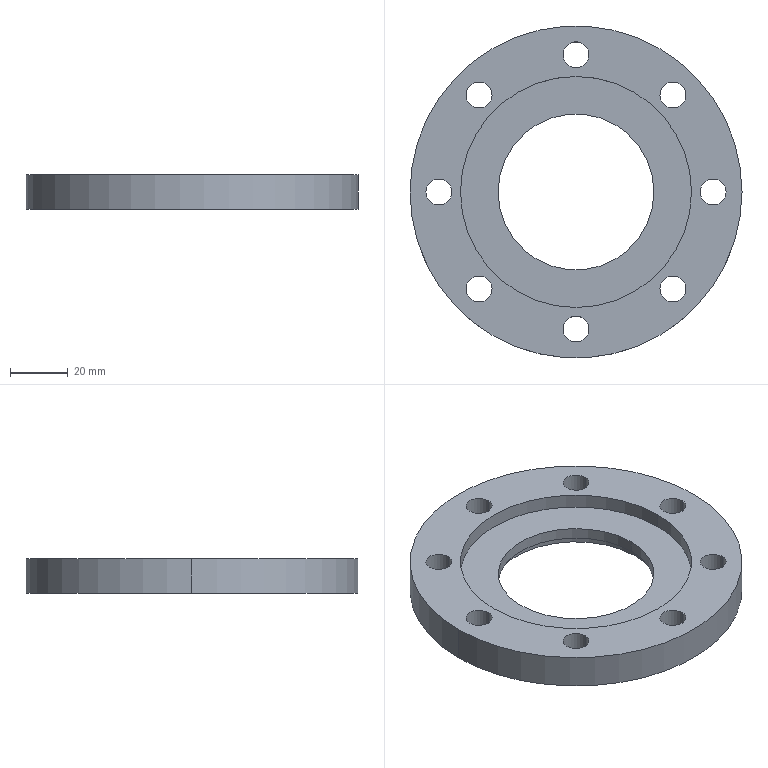Part | SolidWorks | features ICE 4, Extrusion 1 | 1 solid | 28 faces | box 115 x 115 x 12 mm | volume 76316 mm3 | cylinder 24 | plane 4 | commonest cylinder face diameters 9 x16 54 x2 58 x2 80 x2 115 x2
STEP:
#1=CARTESIAN_POINT('',(-4.5,47.5,0.));
#2=VERTEX_POINT('',#1);
#3=CARTESIAN_POINT('',(4.5,47.5,0.));
#4=VERTEX_POINT('',#3);
#5=CARTESIAN_POINT('',(0.,47.5,0.));
#6=DIRECTION('',(0.,0.,1.));
#7=DIRECTION('',(1.,0.,0.));
#8=AXIS2_PLACEMENT_3D('',#5,#6,#7);
#9=CIRCLE('',#8,4.5);
#10=EDGE_CURVE('',#2,#4,#9,.T.);
#11=ORIENTED_EDGE('',*,*,#10,.F.);
#12=CARTESIAN_POINT('',(-4.5,47.5,12.));
#13=VERTEX_POINT('',#12);
#14=CARTESIAN_POINT('',(-4.5,47.5,-38.));
#15=DIRECTION('',(0.,0.,1.));
#16=VECTOR('',#15,1000.);
#17=LINE('',#14,#16);
#18=EDGE_CURVE('',#2,#13,#17,.T.);
#19=ORIENTED_EDGE('',*,*,#18,.T.);
#20=CARTESIAN_POINT('',(4.5,47.5,12.));
#21=VERTEX_POINT('',#20);
#22=CARTESIAN_POINT('',(0.,47.5,12.));
#23=DIRECTION('',(0.,0.,1.));
#24=DIRECTION('',(1.,0.,0.));
#25=AXIS2_PLACEMENT_3D('',#22,#23,#24);
#26=CIRCLE('',#25,4.5);
#27=EDGE_CURVE('',#13,#21,#26,.T.);
#28=ORIENTED_EDGE('',*,*,#27,.T.);
#29=CARTESIAN_POINT('',(4.5,47.5,-38.));
#30=DIRECTION('',(0.,0.,1.));
#31=VECTOR('',#30,1000.);
#32=LINE('',#29,#31);
#33=EDGE_CURVE('',#4,#21,#32,.T.);
#34=ORIENTED_EDGE('',*,*,#33,.F.);
#35=EDGE_LOOP('',(#11,#19,#28,#34));
#36=FACE_OUTER_BOUND('',#35,.T.);
#37=CARTESIAN_POINT('',(0.,47.5,-38.));
#38=DIRECTION('',(0.,0.,1.));
#39=DIRECTION('',(1.,0.,0.));
#40=AXIS2_PLACEMENT_3D('',#37,#38,#39);
#41=CYLINDRICAL_SURFACE('',#40,4.5);
#42=ADVANCED_FACE('',(#36),#41,.F.);
#43=CARTESIAN_POINT('',(29.088,33.588,0.));
#44=VERTEX_POINT('',#43);
#45=CARTESIAN_POINT('',(38.088,33.588,0.));
#46=VERTEX_POINT('',#45);
#47=CARTESIAN_POINT('',(33.588,33.588,0.));
#48=DIRECTION('',(0.,0.,1.));
#49=DIRECTION('',(1.,0.,0.));
#50=AXIS2_PLACEMENT_3D('',#47,#48,#49);
#51=CIRCLE('',#50,4.5);
#52=EDGE_CURVE('',#44,#46,#51,.T.);
#53=ORIENTED_EDGE('',*,*,#52,.F.);
#54=CARTESIAN_POINT('',(29.088,33.588,12.));
#55=VERTEX_POINT('',#54);
#56=CARTESIAN_POINT('',(29.088,33.588,-38.));
#57=DIRECTION('',(0.,0.,1.));
#58=VECTOR('',#57,1000.);
#59=LINE('',#56,#58);
#60=EDGE_CURVE('',#44,#55,#59,.T.);
#61=ORIENTED_EDGE('',*,*,#60,.T.);
#62=CARTESIAN_POINT('',(38.088,33.588,12.));
#63=VERTEX_POINT('',#62);
#64=CARTESIAN_POINT('',(33.588,33.588,12.));
#65=DIRECTION('',(0.,0.,1.));
#66=DIRECTION('',(1.,0.,0.));
#67=AXIS2_PLACEMENT_3D('',#64,#65,#66);
#68=CIRCLE('',#67,4.5);
#69=EDGE_CURVE('',#55,#63,#68,.T.);
#70=ORIENTED_EDGE('',*,*,#69,.T.);
#71=CARTESIAN_POINT('',(38.088,33.588,-38.));
#72=DIRECTION('',(0.,0.,1.));
#73=VECTOR('',#72,1000.);
#74=LINE('',#71,#73);
#75=EDGE_CURVE('',#46,#63,#74,.T.);
#76=ORIENTED_EDGE('',*,*,#75,.F.);
#77=EDGE_LOOP('',(#53,#61,#70,#76));
#78=FACE_OUTER_BOUND('',#77,.T.);
#79=CARTESIAN_POINT('',(33.588,33.588,-38.));
#80=DIRECTION('',(0.,0.,1.));
#81=DIRECTION('',(1.,0.,0.));
#82=AXIS2_PLACEMENT_3D('',#79,#80,#81);
#83=CYLINDRICAL_SURFACE('',#82,4.5);
#84=ADVANCED_FACE('',(#78),#83,.F.);
#85=CARTESIAN_POINT('',(43.,0.,0.));
#86=VERTEX_POINT('',#85);
#87=CARTESIAN_POINT('',(52.,0.,0.));
#88=VERTEX_POINT('',#87);
#89=CARTESIAN_POINT('',(47.5,0.,0.));
#90=DIRECTION('',(0.,0.,1.));
#91=DIRECTION('',(1.,0.,0.));
#92=AXIS2_PLACEMENT_3D('',#89,#90,#91);
#93=CIRCLE('',#92,4.5);
#94=EDGE_CURVE('',#86,#88,#93,.T.);
#95=ORIENTED_EDGE('',*,*,#94,.F.);
#96=CARTESIAN_POINT('',(43.,0.,12.));
#97=VERTEX_POINT('',#96);
#98=CARTESIAN_POINT('',(43.,0.,-38.));
#99=DIRECTION('',(0.,0.,1.));
#100=VECTOR('',#99,1000.);
#101=LINE('',#98,#100);
#102=EDGE_CURVE('',#86,#97,#101,.T.);
#103=ORIENTED_EDGE('',*,*,#102,.T.);
#104=CARTESIAN_POINT('',(52.,0.,12.));
#105=VERTEX_POINT('',#104);
#106=CARTESIAN_POINT('',(47.5,0.,12.));
#107=DIRECTION('',(0.,0.,1.));
#108=DIRECTION('',(1.,0.,0.));
#109=AXIS2_PLACEMENT_3D('',#106,#107,#108);
#110=CIRCLE('',#109,4.5);
#111=EDGE_CURVE('',#97,#105,#110,.T.);
#112=ORIENTED_EDGE('',*,*,#111,.T.);
#113=CARTESIAN_POINT('',(52.,0.,-38.));
#114=DIRECTION('',(0.,0.,1.));
#115=VECTOR('',#114,1000.);
#116=LINE('',#113,#115);
#117=EDGE_CURVE('',#88,#105,#116,.T.);
#118=ORIENTED_EDGE('',*,*,#117,.F.);
#119=EDGE_LOOP('',(#95,#103,#112,#118));
#120=FACE_OUTER_BOUND('',#119,.T.);
#121=CARTESIAN_POINT('',(47.5,0.,-38.));
#122=DIRECTION('',(0.,0.,1.));
#123=DIRECTION('',(1.,0.,0.));
#124=AXIS2_PLACEMENT_3D('',#121,#122,#123);
#125=CYLINDRICAL_SURFACE('',#124,4.5);
#126=ADVANCED_FACE('',(#120),#125,.F.);
#127=CARTESIAN_POINT('',(29.088,-33.588,0.));
#128=VERTEX_POINT('',#127);
#129=CARTESIAN_POINT('',(38.088,-33.588,0.));
#130=VERTEX_POINT('',#129);
#131=CARTESIAN_POINT('',(33.588,-33.588,0.));
#132=DIRECTION('',(0.,0.,1.));
#133=DIRECTION('',(1.,0.,0.));
#134=AXIS2_PLACEMENT_3D('',#131,#132,#133);
#135=CIRCLE('',#134,4.5);
#136=EDGE_CURVE('',#128,#130,#135,.T.);
#137=ORIENTED_EDGE('',*,*,#136,.F.);
#138=CARTESIAN_POINT('',(29.088,-33.588,12.));
#139=VERTEX_POINT('',#138);
#140=CARTESIAN_POINT('',(29.088,-33.588,-38.));
#141=DIRECTION('',(0.,0.,1.));
#142=VECTOR('',#141,1000.);
#143=LINE('',#140,#142);
#144=EDGE_CURVE('',#128,#139,#143,.T.);
#145=ORIENTED_EDGE('',*,*,#144,.T.);
#146=CARTESIAN_POINT('',(38.088,-33.588,12.));
#147=VERTEX_POINT('',#146);
#148=CARTESIAN_POINT('',(33.588,-33.588,12.));
#149=DIRECTION('',(0.,0.,1.));
#150=DIRECTION('',(1.,0.,0.));
#151=AXIS2_PLACEMENT_3D('',#148,#149,#150);
#152=CIRCLE('',#151,4.5);
#153=EDGE_CURVE('',#139,#147,#152,.T.);
#154=ORIENTED_EDGE('',*,*,#153,.T.);
#155=CARTESIAN_POINT('',(38.088,-33.588,-38.));
#156=DIRECTION('',(0.,0.,1.));
#157=VECTOR('',#156,1000.);
#158=LINE('',#155,#157);
#159=EDGE_CURVE('',#130,#147,#158,.T.);
#160=ORIENTED_EDGE('',*,*,#159,.F.);
#161=EDGE_LOOP('',(#137,#145,#154,#160));
#162=FACE_OUTER_BOUND('',#161,.T.);
#163=CARTESIAN_POINT('',(33.588,-33.588,-38.));
#164=DIRECTION('',(0.,0.,1.));
#165=DIRECTION('',(1.,0.,0.));
#166=AXIS2_PLACEMENT_3D('',#163,#164,#165);
#167=CYLINDRICAL_SURFACE('',#166,4.5);
#168=ADVANCED_FACE('',(#162),#167,.F.);
#169=CARTESIAN_POINT('',(-4.5,-47.5,0.));
#170=VERTEX_POINT('',#169);
#171=CARTESIAN_POINT('',(4.5,-47.5,0.));
#172=VERTEX_POINT('',#171);
#173=CARTESIAN_POINT('',(0.,-47.5,0.));
#174=DIRECTION('',(0.,0.,1.));
#175=DIRECTION('',(1.,0.,0.));
#176=AXIS2_PLACEMENT_3D('',#173,#174,#175);
#177=CIRCLE('',#176,4.5);
#178=EDGE_CURVE('',#170,#172,#177,.T.);
#179=ORIENTED_EDGE('',*,*,#178,.F.);
#180=CARTESIAN_POINT('',(-4.5,-47.5,12.));
#181=VERTEX_POINT('',#180);
#182=CARTESIAN_POINT('',(-4.5,-47.5,-38.));
#183=DIRECTION('',(0.,0.,1.));
#184=VECTOR('',#183,1000.);
#185=LINE('',#182,#184);
#186=EDGE_CURVE('',#170,#181,#185,.T.);
#187=ORIENTED_EDGE('',*,*,#186,.T.);
#188=CARTESIAN_POINT('',(4.5,-47.5,12.));
#189=VERTEX_POINT('',#188);
#190=CARTESIAN_POINT('',(0.,-47.5,12.));
#191=DIRECTION('',(0.,0.,1.));
#192=DIRECTION('',(1.,0.,0.));
#193=AXIS2_PLACEMENT_3D('',#190,#191,#192);
#194=CIRCLE('',#193,4.5);
#195=EDGE_CURVE('',#181,#189,#194,.T.);
#196=ORIENTED_EDGE('',*,*,#195,.T.);
#197=CARTESIAN_POINT('',(4.5,-47.5,-38.));
#198=DIRECTION('',(0.,0.,1.));
#199=VECTOR('',#198,1000.);
#200=LINE('',#197,#199);
#201=EDGE_CURVE('',#172,#189,#200,.T.);
#202=ORIENTED_EDGE('',*,*,#201,.F.);
#203=EDGE_LOOP('',(#179,#187,#196,#202));
#204=FACE_OUTER_BOUND('',#203,.T.);
#205=CARTESIAN_POINT('',(0.,-47.5,-38.));
#206=DIRECTION('',(0.,0.,1.));
#207=DIRECTION('',(1.,0.,0.));
#208=AXIS2_PLACEMENT_3D('',#205,#206,#207);
#209=CYLINDRICAL_SURFACE('',#208,4.5);
#210=ADVANCED_FACE('',(#204),#209,.F.);
#211=CARTESIAN_POINT('',(-38.088,-33.588,0.));
#212=VERTEX_POINT('',#211);
#213=CARTESIAN_POINT('',(-29.088,-33.588,0.));
#214=VERTEX_POINT('',#213);
#215=CARTESIAN_POINT('',(-33.588,-33.588,0.));
#216=DIRECTION('',(0.,0.,1.));
#217=DIRECTION('',(1.,0.,0.));
#218=AXIS2_PLACEMENT_3D('',#215,#216,#217);
#219=CIRCLE('',#218,4.5);
#220=EDGE_CURVE('',#212,#214,#219,.T.);
#221=ORIENTED_EDGE('',*,*,#220,.F.);
#222=CARTESIAN_POINT('',(-38.088,-33.588,12.));
#223=VERTEX_POINT('',#222);
#224=CARTESIAN_POINT('',(-38.088,-33.588,-38.));
#225=DIRECTION('',(0.,0.,1.));
#226=VECTOR('',#225,1000.);
#227=LINE('',#224,#226);
#228=EDGE_CURVE('',#212,#223,#227,.T.);
#229=ORIENTED_EDGE('',*,*,#228,.T.);
#230=CARTESIAN_POINT('',(-29.088,-33.588,12.));
#231=VERTEX_POINT('',#230);
#232=CARTESIAN_POINT('',(-33.588,-33.588,12.));
#233=DIRECTION('',(0.,0.,1.));
#234=DIRECTION('',(1.,0.,0.));
#235=AXIS2_PLACEMENT_3D('',#232,#233,#234);
#236=CIRCLE('',#235,4.5);
#237=EDGE_CURVE('',#223,#231,#236,.T.);
#238=ORIENTED_EDGE('',*,*,#237,.T.);
#239=CARTESIAN_POINT('',(-29.088,-33.588,-38.));
#240=DIRECTION('',(0.,0.,1.));
#241=VECTOR('',#240,1000.);
#242=LINE('',#239,#241);
#243=EDGE_CURVE('',#214,#231,#242,.T.);
#244=ORIENTED_EDGE('',*,*,#243,.F.);
#245=EDGE_LOOP('',(#221,#229,#238,#244));
#246=FACE_OUTER_BOUND('',#245,.T.);
#247=CARTESIAN_POINT('',(-33.588,-33.588,-38.));
#248=DIRECTION('',(0.,0.,1.));
#249=DIRECTION('',(1.,0.,0.));
#250=AXIS2_PLACEMENT_3D('',#247,#248,#249);
#251=CYLINDRICAL_SURFACE('',#250,4.5);
#252=ADVANCED_FACE('',(#246),#251,.F.);
#253=CARTESIAN_POINT('',(-52.,0.,0.));
#254=VERTEX_POINT('',#253);
#255=CARTESIAN_POINT('',(-43.,0.,0.));
#256=VERTEX_POINT('',#255);
#257=CARTESIAN_POINT('',(-47.5,0.,0.));
#258=DIRECTION('',(0.,0.,1.));
#259=DIRECTION('',(1.,0.,0.));
#260=AXIS2_PLACEMENT_3D('',#257,#258,#259);
#261=CIRCLE('',#260,4.5);
#262=EDGE_CURVE('',#254,#256,#261,.T.);
#263=ORIENTED_EDGE('',*,*,#262,.F.);
#264=CARTESIAN_POINT('',(-52.,0.,12.));
#265=VERTEX_POINT('',#264);
#266=CARTESIAN_POINT('',(-52.,0.,-38.));
#267=DIRECTION('',(0.,0.,1.));
#268=VECTOR('',#267,1000.);
#269=LINE('',#266,#268);
#270=EDGE_CURVE('',#254,#265,#269,.T.);
#271=ORIENTED_EDGE('',*,*,#270,.T.);
#272=CARTESIAN_POINT('',(-43.,0.,12.));
#273=VERTEX_POINT('',#272);
#274=CARTESIAN_POINT('',(-47.5,0.,12.));
#275=DIRECTION('',(0.,0.,1.));
#276=DIRECTION('',(1.,0.,0.));
#277=AXIS2_PLACEMENT_3D('',#274,#275,#276);
#278=CIRCLE('',#277,4.5);
#279=EDGE_CURVE('',#265,#273,#278,.T.);
#280=ORIENTED_EDGE('',*,*,#279,.T.);
#281=CARTESIAN_POINT('',(-43.,0.,-38.));
#282=DIRECTION('',(0.,0.,1.));
#283=VECTOR('',#282,1000.);
#284=LINE('',#281,#283);
#285=EDGE_CURVE('',#256,#273,#284,.T.);
#286=ORIENTED_EDGE('',*,*,#285,.F.);
#287=EDGE_LOOP('',(#263,#271,#280,#286));
#288=FACE_OUTER_BOUND('',#287,.T.);
#289=CARTESIAN_POINT('',(-47.5,0.,-38.));
#290=DIRECTION('',(0.,0.,1.));
#291=DIRECTION('',(1.,0.,0.));
#292=AXIS2_PLACEMENT_3D('',#289,#290,#291);
#293=CYLINDRICAL_SURFACE('',#292,4.5);
#294=ADVANCED_FACE('',(#288),#293,.F.);
#295=CARTESIAN_POINT('',(-38.088,33.588,0.));
#296=VERTEX_POINT('',#295);
#297=CARTESIAN_POINT('',(-29.088,33.588,0.));
#298=VERTEX_POINT('',#297);
#299=CARTESIAN_POINT('',(-33.588,33.588,0.));
#300=DIRECTION('',(0.,0.,1.));
#301=DIRECTION('',(1.,0.,0.));
#302=AXIS2_PLACEMENT_3D('',#299,#300,#301);
#303=CIRCLE('',#302,4.5);
#304=EDGE_CURVE('',#296,#298,#303,.T.);
#305=ORIENTED_EDGE('',*,*,#304,.F.);
#306=CARTESIAN_POINT('',(-38.088,33.588,12.));
#307=VERTEX_POINT('',#306);
#308=CARTESIAN_POINT('',(-38.088,33.588,-38.));
#309=DIRECTION('',(0.,0.,1.));
#310=VECTOR('',#309,1000.);
#311=LINE('',#308,#310);
#312=EDGE_CURVE('',#296,#307,#311,.T.);
#313=ORIENTED_EDGE('',*,*,#312,.T.);
#314=CARTESIAN_POINT('',(-29.088,33.588,12.));
#315=VERTEX_POINT('',#314);
#316=CARTESIAN_POINT('',(-33.588,33.588,12.));
#317=DIRECTION('',(0.,0.,1.));
#318=DIRECTION('',(1.,0.,0.));
#319=AXIS2_PLACEMENT_3D('',#316,#317,#318);
#320=CIRCLE('',#319,4.5);
#321=EDGE_CURVE('',#307,#315,#320,.T.);
#322=ORIENTED_EDGE('',*,*,#321,.T.);
#323=CARTESIAN_POINT('',(-29.088,33.588,-38.));
#324=DIRECTION('',(0.,0.,1.));
#325=VECTOR('',#324,1000.);
#326=LINE('',#323,#325);
#327=EDGE_CURVE('',#298,#315,#326,.T.);
#328=ORIENTED_EDGE('',*,*,#327,.F.);
#329=EDGE_LOOP('',(#305,#313,#322,#328));
#330=FACE_OUTER_BOUND('',#329,.T.);
#331=CARTESIAN_POINT('',(-33.588,33.588,-38.));
#332=DIRECTION('',(0.,0.,1.));
#333=DIRECTION('',(1.,0.,0.));
#334=AXIS2_PLACEMENT_3D('',#331,#332,#333);
#335=CYLINDRICAL_SURFACE('',#334,4.5);
#336=ADVANCED_FACE('',(#330),#335,.F.);
#337=CARTESIAN_POINT('',(29.,0.,3.));
#338=VERTEX_POINT('',#337);
#339=CARTESIAN_POINT('',(-29.,0.,3.));
#340=VERTEX_POINT('',#339);
#341=CARTESIAN_POINT('',(0.,0.,3.));
#342=DIRECTION('',(0.,0.,-1.));
#343=DIRECTION('',(-1.,0.,0.));
#344=AXIS2_PLACEMENT_3D('',#341,#342,#343);
#345=CIRCLE('',#344,29.);
#346=EDGE_CURVE('',#338,#340,#345,.T.);
#347=ORIENTED_EDGE('',*,*,#346,.F.);
#348=CARTESIAN_POINT('',(29.,0.,0.));
#349=VERTEX_POINT('',#348);
#350=CARTESIAN_POINT('',(29.,0.,3.));
#351=DIRECTION('',(0.,0.,-1.));
#352=VECTOR('',#351,1000.);
#353=LINE('',#350,#352);
#354=EDGE_CURVE('',#338,#349,#353,.T.);
#355=ORIENTED_EDGE('',*,*,#354,.T.);
#356=CARTESIAN_POINT('',(-29.,0.,0.));
#357=VERTEX_POINT('',#356);
#358=CARTESIAN_POINT('',(0.,0.,0.));
#359=DIRECTION('',(0.,0.,-1.));
#360=DIRECTION('',(-1.,0.,0.));
#361=AXIS2_PLACEMENT_3D('',#358,#359,#360);
#362=CIRCLE('',#361,29.);
#363=EDGE_CURVE('',#349,#357,#362,.T.);
#364=ORIENTED_EDGE('',*,*,#363,.T.);
#365=CARTESIAN_POINT('',(-29.,0.,3.));
#366=DIRECTION('',(0.,0.,-1.));
#367=VECTOR('',#366,1000.);
#368=LINE('',#365,#367);
#369=EDGE_CURVE('',#340,#357,#368,.T.);
#370=ORIENTED_EDGE('',*,*,#369,.F.);
#371=EDGE_LOOP('',(#347,#355,#364,#370));
#372=FACE_OUTER_BOUND('',#371,.T.);
#373=CARTESIAN_POINT('',(0.,0.,3.));
#374=DIRECTION('',(0.,0.,-1.));
#375=DIRECTION('',(-1.,0.,0.));
#376=AXIS2_PLACEMENT_3D('',#373,#374,#375);
#377=CYLINDRICAL_SURFACE('',#376,29.);
#378=ADVANCED_FACE('',(#372),#377,.F.);
#379=CARTESIAN_POINT('',(-40.,0.,7.));
#380=VERTEX_POINT('',#379);
#381=CARTESIAN_POINT('',(40.,0.,7.));
#382=VERTEX_POINT('',#381);
#383=CARTESIAN_POINT('',(0.,0.,7.));
#384=DIRECTION('',(0.,0.,1.));
#385=DIRECTION('',(1.,0.,0.));
#386=AXIS2_PLACEMENT_3D('',#383,#384,#385);
#387=CIRCLE('',#386,40.);
#388=EDGE_CURVE('',#380,#382,#387,.T.);
#389=ORIENTED_EDGE('',*,*,#388,.F.);
#390=CARTESIAN_POINT('',(-40.,0.,12.));
#391=VERTEX_POINT('',#390);
#392=CARTESIAN_POINT('',(-40.,0.,7.));
#393=DIRECTION('',(0.,0.,1.));
#394=VECTOR('',#393,1000.);
#395=LINE('',#392,#394);
#396=EDGE_CURVE('',#380,#391,#395,.T.);
#397=ORIENTED_EDGE('',*,*,#396,.T.);
#398=CARTESIAN_POINT('',(40.,0.,12.));
#399=VERTEX_POINT('',#398);
#400=CARTESIAN_POINT('',(0.,0.,12.));
#401=DIRECTION('',(0.,0.,1.));
#402=DIRECTION('',(1.,0.,0.));
#403=AXIS2_PLACEMENT_3D('',#400,#401,#402);
#404=CIRCLE('',#403,40.);
#405=EDGE_CURVE('',#391,#399,#404,.T.);
#406=ORIENTED_EDGE('',*,*,#405,.T.);
#407=CARTESIAN_POINT('',(40.,0.,7.));
#408=DIRECTION('',(0.,0.,1.));
#409=VECTOR('',#408,1000.);
#410=LINE('',#407,#409);
#411=EDGE_CURVE('',#382,#399,#410,.T.);
#412=ORIENTED_EDGE('',*,*,#411,.F.);
#413=EDGE_LOOP('',(#389,#397,#406,#412));
#414=FACE_OUTER_BOUND('',#413,.T.);
#415=CARTESIAN_POINT('',(0.,0.,7.));
#416=DIRECTION('',(0.,0.,1.));
#417=DIRECTION('',(1.,0.,0.));
#418=AXIS2_PLACEMENT_3D('',#415,#416,#417);
#419=CYLINDRICAL_SURFACE('',#418,40.);
#420=ADVANCED_FACE('',(#414),#419,.F.);
#421=CARTESIAN_POINT('',(57.5,0.,12.));
#422=VERTEX_POINT('',#421);
#423=CARTESIAN_POINT('',(-57.5,0.,12.));
#424=VERTEX_POINT('',#423);
#425=CARTESIAN_POINT('',(0.,0.,12.));
#426=DIRECTION('',(0.,0.,1.));
#427=DIRECTION('',(1.,0.,0.));
#428=AXIS2_PLACEMENT_3D('',#425,#426,#427);
#429=CIRCLE('',#428,57.5);
#430=EDGE_CURVE('',#422,#424,#429,.T.);
#431=ORIENTED_EDGE('',*,*,#430,.F.);
#432=CARTESIAN_POINT('',(57.5,0.,0.));
#433=VERTEX_POINT('',#432);
#434=CARTESIAN_POINT('',(57.5,0.,12.));
#435=DIRECTION('',(0.,0.,-1.));
#436=VECTOR('',#435,1000.);
#437=LINE('',#434,#436);
#438=EDGE_CURVE('',#422,#433,#437,.T.);
#439=ORIENTED_EDGE('',*,*,#438,.T.);
#440=CARTESIAN_POINT('',(-57.5,0.,0.));
#441=VERTEX_POINT('',#440);
#442=CARTESIAN_POINT('',(0.,0.,0.));
#443=DIRECTION('',(0.,0.,1.));
#444=DIRECTION('',(1.,0.,0.));
#445=AXIS2_PLACEMENT_3D('',#442,#443,#444);
#446=CIRCLE('',#445,57.5);
#447=EDGE_CURVE('',#433,#441,#446,.T.);
#448=ORIENTED_EDGE('',*,*,#447,.T.);
#449=CARTESIAN_POINT('',(-57.5,0.,12.));
#450=DIRECTION('',(0.,0.,-1.));
#451=VECTOR('',#450,1000.);
#452=LINE('',#449,#451);
#453=EDGE_CURVE('',#424,#441,#452,.T.);
#454=ORIENTED_EDGE('',*,*,#453,.F.);
#455=EDGE_LOOP('',(#431,#439,#448,#454));
#456=FACE_OUTER_BOUND('',#455,.T.);
#457=CARTESIAN_POINT('',(0.,0.,12.));
#458=DIRECTION('',(0.,0.,-1.));
#459=DIRECTION('',(-1.,0.,0.));
#460=AXIS2_PLACEMENT_3D('',#457,#458,#459);
#461=CYLINDRICAL_SURFACE('',#460,57.5);
#462=ADVANCED_FACE('',(#456),#461,.T.);
#463=CARTESIAN_POINT('',(-27.,0.,3.));
#464=VERTEX_POINT('',#463);
#465=CARTESIAN_POINT('',(27.,0.,3.));
#466=VERTEX_POINT('',#465);
#467=CARTESIAN_POINT('',(0.,0.,3.));
#468=DIRECTION('',(0.,0.,1.));
#469=DIRECTION('',(-1.,0.,0.));
#470=AXIS2_PLACEMENT_3D('',#467,#468,#469);
#471=CIRCLE('',#470,27.);
#472=EDGE_CURVE('',#464,#466,#471,.T.);
#473=ORIENTED_EDGE('',*,*,#472,.F.);
#474=CARTESIAN_POINT('',(-27.,0.,7.));
#475=VERTEX_POINT('',#474);
#476=CARTESIAN_POINT('',(-27.,0.,-6.));
#477=DIRECTION('',(0.,0.,1.));
#478=VECTOR('',#477,1000.);
#479=LINE('',#476,#478);
#480=EDGE_CURVE('',#464,#475,#479,.T.);
#481=ORIENTED_EDGE('',*,*,#480,.T.);
#482=CARTESIAN_POINT('',(27.,0.,7.));
#483=VERTEX_POINT('',#482);
#484=CARTESIAN_POINT('',(0.,0.,7.));
#485=DIRECTION('',(0.,0.,1.));
#486=DIRECTION('',(1.,0.,0.));
#487=AXIS2_PLACEMENT_3D('',#484,#485,#486);
#488=CIRCLE('',#487,27.);
#489=EDGE_CURVE('',#475,#483,#488,.T.);
#490=ORIENTED_EDGE('',*,*,#489,.T.);
#491=CARTESIAN_POINT('',(27.,0.,-6.));
#492=DIRECTION('',(0.,0.,1.));
#493=VECTOR('',#492,1000.);
#494=LINE('',#491,#493);
#495=EDGE_CURVE('',#466,#483,#494,.T.);
#496=ORIENTED_EDGE('',*,*,#495,.F.);
#497=EDGE_LOOP('',(#473,#481,#490,#496));
#498=FACE_OUTER_BOUND('',#497,.T.);
#499=CARTESIAN_POINT('',(0.,0.,-6.));
#500=DIRECTION('',(0.,0.,1.));
#501=DIRECTION('',(1.,0.,0.));
#502=AXIS2_PLACEMENT_3D('',#499,#500,#501);
#503=CYLINDRICAL_SURFACE('',#502,27.);
#504=ADVANCED_FACE('',(#498),#503,.F.);
#505=ORIENTED_EDGE('',*,*,#480,.F.);
#506=CARTESIAN_POINT('',(0.,0.,3.));
#507=DIRECTION('',(0.,0.,1.));
#508=DIRECTION('',(-1.,0.,0.));
#509=AXIS2_PLACEMENT_3D('',#506,#507,#508);
#510=CIRCLE('',#509,27.);
#511=EDGE_CURVE('',#466,#464,#510,.T.);
#512=ORIENTED_EDGE('',*,*,#511,.F.);
#513=ORIENTED_EDGE('',*,*,#495,.T.);
#514=CARTESIAN_POINT('',(0.,0.,7.));
#515=DIRECTION('',(0.,0.,1.));
#516=DIRECTION('',(1.,0.,0.));
#517=AXIS2_PLACEMENT_3D('',#514,#515,#516);
#518=CIRCLE('',#517,27.);
#519=EDGE_CURVE('',#483,#475,#518,.T.);
#520=ORIENTED_EDGE('',*,*,#519,.T.);
#521=EDGE_LOOP('',(#505,#512,#513,#520));
#522=FACE_OUTER_BOUND('',#521,.T.);
#523=CARTESIAN_POINT('',(0.,0.,-6.));
#524=DIRECTION('',(0.,0.,1.));
#525=DIRECTION('',(1.,0.,0.));
#526=AXIS2_PLACEMENT_3D('',#523,#524,#525);
#527=CYLINDRICAL_SURFACE('',#526,27.);
#528=ADVANCED_FACE('',(#522),#527,.F.);
#529=ORIENTED_EDGE('',*,*,#438,.F.);
#530=CARTESIAN_POINT('',(0.,0.,12.));
#531=DIRECTION('',(0.,0.,1.));
#532=DIRECTION('',(1.,0.,0.));
#533=AXIS2_PLACEMENT_3D('',#530,#531,#532);
#534=CIRCLE('',#533,57.5);
#535=EDGE_CURVE('',#424,#422,#534,.T.);
#536=ORIENTED_EDGE('',*,*,#535,.F.);
#537=ORIENTED_EDGE('',*,*,#453,.T.);
#538=CARTESIAN_POINT('',(0.,0.,0.));
#539=DIRECTION('',(0.,0.,1.));
#540=DIRECTION('',(1.,0.,0.));
#541=AXIS2_PLACEMENT_3D('',#538,#539,#540);
#542=CIRCLE('',#541,57.5);
#543=EDGE_CURVE('',#441,#433,#542,.T.);
#544=ORIENTED_EDGE('',*,*,#543,.T.);
#545=EDGE_LOOP('',(#529,#536,#537,#544));
#546=FACE_OUTER_BOUND('',#545,.T.);
#547=CARTESIAN_POINT('',(0.,0.,12.));
#548=DIRECTION('',(0.,0.,-1.));
#549=DIRECTION('',(-1.,0.,0.));
#550=AXIS2_PLACEMENT_3D('',#547,#548,#549);
#551=CYLINDRICAL_SURFACE('',#550,57.5);
#552=ADVANCED_FACE('',(#546),#551,.T.);
#553=CARTESIAN_POINT('',(0.,47.5,12.));
#554=DIRECTION('',(0.,0.,1.));
#555=DIRECTION('',(1.,0.,0.));
#556=AXIS2_PLACEMENT_3D('',#553,#554,#555);
#557=CIRCLE('',#556,4.5);
#558=EDGE_CURVE('',#21,#13,#557,.T.);
#559=ORIENTED_EDGE('',*,*,#558,.F.);
#560=ORIENTED_EDGE('',*,*,#27,.F.);
#561=EDGE_LOOP('',(#559,#560));
#562=FACE_BOUND('',#561,.T.);
#563=CARTESIAN_POINT('',(33.588,33.588,12.));
#564=DIRECTION('',(0.,0.,1.));
#565=DIRECTION('',(1.,0.,0.));
#566=AXIS2_PLACEMENT_3D('',#563,#564,#565);
#567=CIRCLE('',#566,4.5);
#568=EDGE_CURVE('',#63,#55,#567,.T.);
#569=ORIENTED_EDGE('',*,*,#568,.F.);
#570=ORIENTED_EDGE('',*,*,#69,.F.);
#571=EDGE_LOOP('',(#569,#570));
#572=FACE_BOUND('',#571,.T.);
#573=CARTESIAN_POINT('',(47.5,0.,12.));
#574=DIRECTION('',(0.,0.,1.));
#575=DIRECTION('',(1.,0.,0.));
#576=AXIS2_PLACEMENT_3D('',#573,#574,#575);
#577=CIRCLE('',#576,4.5);
#578=EDGE_CURVE('',#105,#97,#577,.T.);
#579=ORIENTED_EDGE('',*,*,#578,.F.);
#580=ORIENTED_EDGE('',*,*,#111,.F.);
#581=EDGE_LOOP('',(#579,#580));
#582=FACE_BOUND('',#581,.T.);
#583=CARTESIAN_POINT('',(33.588,-33.588,12.));
#584=DIRECTION('',(0.,0.,1.));
#585=DIRECTION('',(1.,0.,0.));
#586=AXIS2_PLACEMENT_3D('',#583,#584,#585);
#587=CIRCLE('',#586,4.5);
#588=EDGE_CURVE('',#147,#139,#587,.T.);
#589=ORIENTED_EDGE('',*,*,#588,.F.);
#590=ORIENTED_EDGE('',*,*,#153,.F.);
#591=EDGE_LOOP('',(#589,#590));
#592=FACE_BOUND('',#591,.T.);
#593=CARTESIAN_POINT('',(0.,-47.5,12.));
#594=DIRECTION('',(0.,0.,1.));
#595=DIRECTION('',(1.,0.,0.));
#596=AXIS2_PLACEMENT_3D('',#593,#594,#595);
#597=CIRCLE('',#596,4.5);
#598=EDGE_CURVE('',#189,#181,#597,.T.);
#599=ORIENTED_EDGE('',*,*,#598,.F.);
#600=ORIENTED_EDGE('',*,*,#195,.F.);
#601=EDGE_LOOP('',(#599,#600));
#602=FACE_BOUND('',#601,.T.);
#603=CARTESIAN_POINT('',(-33.588,-33.588,12.));
#604=DIRECTION('',(0.,0.,1.));
#605=DIRECTION('',(1.,0.,0.));
#606=AXIS2_PLACEMENT_3D('',#603,#604,#605);
#607=CIRCLE('',#606,4.5);
#608=EDGE_CURVE('',#231,#223,#607,.T.);
#609=ORIENTED_EDGE('',*,*,#608,.F.);
#610=ORIENTED_EDGE('',*,*,#237,.F.);
#611=EDGE_LOOP('',(#609,#610));
#612=FACE_BOUND('',#611,.T.);
#613=CARTESIAN_POINT('',(-47.5,0.,12.));
#614=DIRECTION('',(0.,0.,1.));
#615=DIRECTION('',(1.,0.,0.));
#616=AXIS2_PLACEMENT_3D('',#613,#614,#615);
#617=CIRCLE('',#616,4.5);
#618=EDGE_CURVE('',#273,#265,#617,.T.);
#619=ORIENTED_EDGE('',*,*,#618,.F.);
#620=ORIENTED_EDGE('',*,*,#279,.F.);
#621=EDGE_LOOP('',(#619,#620));
#622=FACE_BOUND('',#621,.T.);
#623=CARTESIAN_POINT('',(-33.588,33.588,12.));
#624=DIRECTION('',(0.,0.,1.));
#625=DIRECTION('',(1.,0.,0.));
#626=AXIS2_PLACEMENT_3D('',#623,#624,#625);
#627=CIRCLE('',#626,4.5);
#628=EDGE_CURVE('',#315,#307,#627,.T.);
#629=ORIENTED_EDGE('',*,*,#628,.F.);
#630=ORIENTED_EDGE('',*,*,#321,.F.);
#631=EDGE_LOOP('',(#629,#630));
#632=FACE_BOUND('',#631,.T.);
#633=CARTESIAN_POINT('',(0.,0.,12.));
#634=DIRECTION('',(0.,0.,1.));
#635=DIRECTION('',(1.,0.,0.));
#636=AXIS2_PLACEMENT_3D('',#633,#634,#635);
#637=CIRCLE('',#636,40.);
#638=EDGE_CURVE('',#399,#391,#637,.T.);
#639=ORIENTED_EDGE('',*,*,#638,.F.);
#640=ORIENTED_EDGE('',*,*,#405,.F.);
#641=EDGE_LOOP('',(#639,#640));
#642=FACE_BOUND('',#641,.T.);
#643=ORIENTED_EDGE('',*,*,#535,.T.);
#644=ORIENTED_EDGE('',*,*,#430,.T.);
#645=EDGE_LOOP('',(#643,#644));
#646=FACE_OUTER_BOUND('',#645,.T.);
#647=CARTESIAN_POINT('',(0.,0.,12.));
#648=DIRECTION('',(0.,0.,1.));
#649=DIRECTION('',(1.,0.,0.));
#650=AXIS2_PLACEMENT_3D('',#647,#648,#649);
#651=PLANE('',#650);
#652=ADVANCED_FACE('',(#562,#572,#582,#592,#602,#612,#622,#632,#642,#646),#651,.T.);
#653=CARTESIAN_POINT('',(0.,47.5,0.));
#654=DIRECTION('',(0.,0.,1.));
#655=DIRECTION('',(1.,0.,0.));
#656=AXIS2_PLACEMENT_3D('',#653,#654,#655);
#657=CIRCLE('',#656,4.5);
#658=EDGE_CURVE('',#4,#2,#657,.T.);
#659=ORIENTED_EDGE('',*,*,#658,.T.);
#660=ORIENTED_EDGE('',*,*,#10,.T.);
#661=EDGE_LOOP('',(#659,#660));
#662=FACE_BOUND('',#661,.T.);
#663=CARTESIAN_POINT('',(33.588,33.588,0.));
#664=DIRECTION('',(0.,0.,1.));
#665=DIRECTION('',(1.,0.,0.));
#666=AXIS2_PLACEMENT_3D('',#663,#664,#665);
#667=CIRCLE('',#666,4.5);
#668=EDGE_CURVE('',#46,#44,#667,.T.);
#669=ORIENTED_EDGE('',*,*,#668,.T.);
#670=ORIENTED_EDGE('',*,*,#52,.T.);
#671=EDGE_LOOP('',(#669,#670));
#672=FACE_BOUND('',#671,.T.);
#673=CARTESIAN_POINT('',(47.5,0.,0.));
#674=DIRECTION('',(0.,0.,1.));
#675=DIRECTION('',(1.,0.,0.));
#676=AXIS2_PLACEMENT_3D('',#673,#674,#675);
#677=CIRCLE('',#676,4.5);
#678=EDGE_CURVE('',#88,#86,#677,.T.);
#679=ORIENTED_EDGE('',*,*,#678,.T.);
#680=ORIENTED_EDGE('',*,*,#94,.T.);
#681=EDGE_LOOP('',(#679,#680));
#682=FACE_BOUND('',#681,.T.);
#683=CARTESIAN_POINT('',(33.588,-33.588,0.));
#684=DIRECTION('',(0.,0.,1.));
#685=DIRECTION('',(1.,0.,0.));
#686=AXIS2_PLACEMENT_3D('',#683,#684,#685);
#687=CIRCLE('',#686,4.5);
#688=EDGE_CURVE('',#130,#128,#687,.T.);
#689=ORIENTED_EDGE('',*,*,#688,.T.);
#690=ORIENTED_EDGE('',*,*,#136,.T.);
#691=EDGE_LOOP('',(#689,#690));
#692=FACE_BOUND('',#691,.T.);
#693=CARTESIAN_POINT('',(0.,-47.5,0.));
#694=DIRECTION('',(0.,0.,1.));
#695=DIRECTION('',(1.,0.,0.));
#696=AXIS2_PLACEMENT_3D('',#693,#694,#695);
#697=CIRCLE('',#696,4.5);
#698=EDGE_CURVE('',#172,#170,#697,.T.);
#699=ORIENTED_EDGE('',*,*,#698,.T.);
#700=ORIENTED_EDGE('',*,*,#178,.T.);
#701=EDGE_LOOP('',(#699,#700));
#702=FACE_BOUND('',#701,.T.);
#703=CARTESIAN_POINT('',(-33.588,-33.588,0.));
#704=DIRECTION('',(0.,0.,1.));
#705=DIRECTION('',(1.,0.,0.));
#706=AXIS2_PLACEMENT_3D('',#703,#704,#705);
#707=CIRCLE('',#706,4.5);
#708=EDGE_CURVE('',#214,#212,#707,.T.);
#709=ORIENTED_EDGE('',*,*,#708,.T.);
#710=ORIENTED_EDGE('',*,*,#220,.T.);
#711=EDGE_LOOP('',(#709,#710));
#712=FACE_BOUND('',#711,.T.);
#713=CARTESIAN_POINT('',(-47.5,0.,0.));
#714=DIRECTION('',(0.,0.,1.));
#715=DIRECTION('',(1.,0.,0.));
#716=AXIS2_PLACEMENT_3D('',#713,#714,#715);
#717=CIRCLE('',#716,4.5);
#718=EDGE_CURVE('',#256,#254,#717,.T.);
#719=ORIENTED_EDGE('',*,*,#718,.T.);
#720=ORIENTED_EDGE('',*,*,#262,.T.);
#721=EDGE_LOOP('',(#719,#720));
#722=FACE_BOUND('',#721,.T.);
#723=CARTESIAN_POINT('',(-33.588,33.588,0.));
#724=DIRECTION('',(0.,0.,1.));
#725=DIRECTION('',(1.,0.,0.));
#726=AXIS2_PLACEMENT_3D('',#723,#724,#725);
#727=CIRCLE('',#726,4.5);
#728=EDGE_CURVE('',#298,#296,#727,.T.);
#729=ORIENTED_EDGE('',*,*,#728,.T.);
#730=ORIENTED_EDGE('',*,*,#304,.T.);
#731=EDGE_LOOP('',(#729,#730));
#732=FACE_BOUND('',#731,.T.);
#733=CARTESIAN_POINT('',(0.,0.,0.));
#734=DIRECTION('',(0.,0.,-1.));
#735=DIRECTION('',(-1.,0.,0.));
#736=AXIS2_PLACEMENT_3D('',#733,#734,#735);
#737=CIRCLE('',#736,29.);
#738=EDGE_CURVE('',#357,#349,#737,.T.);
#739=ORIENTED_EDGE('',*,*,#738,.F.);
#740=ORIENTED_EDGE('',*,*,#363,.F.);
#741=EDGE_LOOP('',(#739,#740));
#742=FACE_BOUND('',#741,.T.);
#743=ORIENTED_EDGE('',*,*,#543,.F.);
#744=ORIENTED_EDGE('',*,*,#447,.F.);
#745=EDGE_LOOP('',(#743,#744));
#746=FACE_OUTER_BOUND('',#745,.T.);
#747=CARTESIAN_POINT('',(0.,0.,0.));
#748=DIRECTION('',(0.,0.,1.));
#749=DIRECTION('',(1.,0.,0.));
#750=AXIS2_PLACEMENT_3D('',#747,#748,#749);
#751=PLANE('',#750);
#752=ADVANCED_FACE('',(#662,#672,#682,#692,#702,#712,#722,#732,#742,#746),#751,.F.);
#753=ORIENTED_EDGE('',*,*,#396,.F.);
#754=CARTESIAN_POINT('',(0.,0.,7.));
#755=DIRECTION('',(0.,0.,1.));
#756=DIRECTION('',(1.,0.,0.));
#757=AXIS2_PLACEMENT_3D('',#754,#755,#756);
#758=CIRCLE('',#757,40.);
#759=EDGE_CURVE('',#382,#380,#758,.T.);
#760=ORIENTED_EDGE('',*,*,#759,.F.);
#761=ORIENTED_EDGE('',*,*,#411,.T.);
#762=ORIENTED_EDGE('',*,*,#638,.T.);
#763=EDGE_LOOP('',(#753,#760,#761,#762));
#764=FACE_OUTER_BOUND('',#763,.T.);
#765=CARTESIAN_POINT('',(0.,0.,7.));
#766=DIRECTION('',(0.,0.,1.));
#767=DIRECTION('',(1.,0.,0.));
#768=AXIS2_PLACEMENT_3D('',#765,#766,#767);
#769=CYLINDRICAL_SURFACE('',#768,40.);
#770=ADVANCED_FACE('',(#764),#769,.F.);
#771=ORIENTED_EDGE('',*,*,#519,.F.);
#772=ORIENTED_EDGE('',*,*,#489,.F.);
#773=EDGE_LOOP('',(#771,#772));
#774=FACE_BOUND('',#773,.T.);
#775=ORIENTED_EDGE('',*,*,#759,.T.);
#776=ORIENTED_EDGE('',*,*,#388,.T.);
#777=EDGE_LOOP('',(#775,#776));
#778=FACE_OUTER_BOUND('',#777,.T.);
#779=CARTESIAN_POINT('',(0.,0.,7.));
#780=DIRECTION('',(0.,0.,1.));
#781=DIRECTION('',(1.,0.,0.));
#782=AXIS2_PLACEMENT_3D('',#779,#780,#781);
#783=PLANE('',#782);
#784=ADVANCED_FACE('',(#774,#778),#783,.T.);
#785=CARTESIAN_POINT('',(0.,0.,3.));
#786=DIRECTION('',(0.,0.,-1.));
#787=DIRECTION('',(-1.,0.,0.));
#788=AXIS2_PLACEMENT_3D('',#785,#786,#787);
#789=CIRCLE('',#788,29.);
#790=EDGE_CURVE('',#340,#338,#789,.T.);
#791=ORIENTED_EDGE('',*,*,#790,.T.);
#792=ORIENTED_EDGE('',*,*,#346,.T.);
#793=EDGE_LOOP('',(#791,#792));
#794=FACE_OUTER_BOUND('',#793,.T.);
#795=ORIENTED_EDGE('',*,*,#511,.T.);
#796=ORIENTED_EDGE('',*,*,#472,.T.);
#797=EDGE_LOOP('',(#795,#796));
#798=FACE_BOUND('',#797,.T.);
#799=CARTESIAN_POINT('',(0.,0.,3.));
#800=DIRECTION('',(0.,0.,-1.));
#801=DIRECTION('',(-1.,0.,0.));
#802=AXIS2_PLACEMENT_3D('',#799,#800,#801);
#803=PLANE('',#802);
#804=ADVANCED_FACE('',(#794,#798),#803,.T.);
#805=ORIENTED_EDGE('',*,*,#354,.F.);
#806=ORIENTED_EDGE('',*,*,#790,.F.);
#807=ORIENTED_EDGE('',*,*,#369,.T.);
#808=ORIENTED_EDGE('',*,*,#738,.T.);
#809=EDGE_LOOP('',(#805,#806,#807,#808));
#810=FACE_OUTER_BOUND('',#809,.T.);
#811=CARTESIAN_POINT('',(0.,0.,3.));
#812=DIRECTION('',(0.,0.,-1.));
#813=DIRECTION('',(-1.,0.,0.));
#814=AXIS2_PLACEMENT_3D('',#811,#812,#813);
#815=CYLINDRICAL_SURFACE('',#814,29.);
#816=ADVANCED_FACE('',(#810),#815,.F.);
#817=ORIENTED_EDGE('',*,*,#312,.F.);
#818=ORIENTED_EDGE('',*,*,#728,.F.);
#819=ORIENTED_EDGE('',*,*,#327,.T.);
#820=ORIENTED_EDGE('',*,*,#628,.T.);
#821=EDGE_LOOP('',(#817,#818,#819,#820));
#822=FACE_OUTER_BOUND('',#821,.T.);
#823=CARTESIAN_POINT('',(-33.588,33.588,-38.));
#824=DIRECTION('',(0.,0.,1.));
#825=DIRECTION('',(1.,0.,0.));
#826=AXIS2_PLACEMENT_3D('',#823,#824,#825);
#827=CYLINDRICAL_SURFACE('',#826,4.5);
#828=ADVANCED_FACE('',(#822),#827,.F.);
#829=ORIENTED_EDGE('',*,*,#270,.F.);
#830=ORIENTED_EDGE('',*,*,#718,.F.);
#831=ORIENTED_EDGE('',*,*,#285,.T.);
#832=ORIENTED_EDGE('',*,*,#618,.T.);
#833=EDGE_LOOP('',(#829,#830,#831,#832));
#834=FACE_OUTER_BOUND('',#833,.T.);
#835=CARTESIAN_POINT('',(-47.5,0.,-38.));
#836=DIRECTION('',(0.,0.,1.));
#837=DIRECTION('',(1.,0.,0.));
#838=AXIS2_PLACEMENT_3D('',#835,#836,#837);
#839=CYLINDRICAL_SURFACE('',#838,4.5);
#840=ADVANCED_FACE('',(#834),#839,.F.);
#841=ORIENTED_EDGE('',*,*,#228,.F.);
#842=ORIENTED_EDGE('',*,*,#708,.F.);
#843=ORIENTED_EDGE('',*,*,#243,.T.);
#844=ORIENTED_EDGE('',*,*,#608,.T.);
#845=EDGE_LOOP('',(#841,#842,#843,#844));
#846=FACE_OUTER_BOUND('',#845,.T.);
#847=CARTESIAN_POINT('',(-33.588,-33.588,-38.));
#848=DIRECTION('',(0.,0.,1.));
#849=DIRECTION('',(1.,0.,0.));
#850=AXIS2_PLACEMENT_3D('',#847,#848,#849);
#851=CYLINDRICAL_SURFACE('',#850,4.5);
#852=ADVANCED_FACE('',(#846),#851,.F.);
#853=ORIENTED_EDGE('',*,*,#186,.F.);
#854=ORIENTED_EDGE('',*,*,#698,.F.);
#855=ORIENTED_EDGE('',*,*,#201,.T.);
#856=ORIENTED_EDGE('',*,*,#598,.T.);
#857=EDGE_LOOP('',(#853,#854,#855,#856));
#858=FACE_OUTER_BOUND('',#857,.T.);
#859=CARTESIAN_POINT('',(0.,-47.5,-38.));
#860=DIRECTION('',(0.,0.,1.));
#861=DIRECTION('',(1.,0.,0.));
#862=AXIS2_PLACEMENT_3D('',#859,#860,#861);
#863=CYLINDRICAL_SURFACE('',#862,4.5);
#864=ADVANCED_FACE('',(#858),#863,.F.);
#865=ORIENTED_EDGE('',*,*,#144,.F.);
#866=ORIENTED_EDGE('',*,*,#688,.F.);
#867=ORIENTED_EDGE('',*,*,#159,.T.);
#868=ORIENTED_EDGE('',*,*,#588,.T.);
#869=EDGE_LOOP('',(#865,#866,#867,#868));
#870=FACE_OUTER_BOUND('',#869,.T.);
#871=CARTESIAN_POINT('',(33.588,-33.588,-38.));
#872=DIRECTION('',(0.,0.,1.));
#873=DIRECTION('',(1.,0.,0.));
#874=AXIS2_PLACEMENT_3D('',#871,#872,#873);
#875=CYLINDRICAL_SURFACE('',#874,4.5);
#876=ADVANCED_FACE('',(#870),#875,.F.);
#877=ORIENTED_EDGE('',*,*,#102,.F.);
#878=ORIENTED_EDGE('',*,*,#678,.F.);
#879=ORIENTED_EDGE('',*,*,#117,.T.);
#880=ORIENTED_EDGE('',*,*,#578,.T.);
#881=EDGE_LOOP('',(#877,#878,#879,#880));
#882=FACE_OUTER_BOUND('',#881,.T.);
#883=CARTESIAN_POINT('',(47.5,0.,-38.));
#884=DIRECTION('',(0.,0.,1.));
#885=DIRECTION('',(1.,0.,0.));
#886=AXIS2_PLACEMENT_3D('',#883,#884,#885);
#887=CYLINDRICAL_SURFACE('',#886,4.5);
#888=ADVANCED_FACE('',(#882),#887,.F.);
#889=ORIENTED_EDGE('',*,*,#60,.F.);
#890=ORIENTED_EDGE('',*,*,#668,.F.);
#891=ORIENTED_EDGE('',*,*,#75,.T.);
#892=ORIENTED_EDGE('',*,*,#568,.T.);
#893=EDGE_LOOP('',(#889,#890,#891,#892));
#894=FACE_OUTER_BOUND('',#893,.T.);
#895=CARTESIAN_POINT('',(33.588,33.588,-38.));
#896=DIRECTION('',(0.,0.,1.));
#897=DIRECTION('',(1.,0.,0.));
#898=AXIS2_PLACEMENT_3D('',#895,#896,#897);
#899=CYLINDRICAL_SURFACE('',#898,4.5);
#900=ADVANCED_FACE('',(#894),#899,.F.);
#901=ORIENTED_EDGE('',*,*,#18,.F.);
#902=ORIENTED_EDGE('',*,*,#658,.F.);
#903=ORIENTED_EDGE('',*,*,#33,.T.);
#904=ORIENTED_EDGE('',*,*,#558,.T.);
#905=EDGE_LOOP('',(#901,#902,#903,#904));
#906=FACE_OUTER_BOUND('',#905,.T.);
#907=CARTESIAN_POINT('',(0.,47.5,-38.));
#908=DIRECTION('',(0.,0.,1.));
#909=DIRECTION('',(1.,0.,0.));
#910=AXIS2_PLACEMENT_3D('',#907,#908,#909);
#911=CYLINDRICAL_SURFACE('',#910,4.5);
#912=ADVANCED_FACE('',(#906),#911,.F.);
#913=CLOSED_SHELL('',(#42,#84,#126,#168,#210,#252,#294,#336,#378,#420,#462,#504,#528,#552,#652,#752,#770,#784,#804,#816,#828,#840,#852,#864,#876,#888,#900,#912));
#914=MANIFOLD_SOLID_BREP('',#913);
#915=CARTESIAN_POINT('',(0.,0.,0.));
#916=DIRECTION('',(0.,0.,1.));
#917=DIRECTION('',(1.,0.,0.));
#918=AXIS2_PLACEMENT_3D('',#915,#916,#917);
#919=(LENGTH_UNIT()NAMED_UNIT(*)SI_UNIT(.MILLI.,.METRE.));
#920=UNCERTAINTY_MEASURE_WITH_UNIT(LENGTH_MEASURE(0.00001),#919,'','');
#921=(NAMED_UNIT(*)PLANE_ANGLE_UNIT()SI_UNIT($,.RADIAN.));
#922=(NAMED_UNIT(*)SI_UNIT($,.STERADIAN.)SOLID_ANGLE_UNIT());
#923=(GEOMETRIC_REPRESENTATION_CONTEXT(3)GLOBAL_UNCERTAINTY_ASSIGNED_CONTEXT((#920))GLOBAL_UNIT_ASSIGNED_CONTEXT((#919,#921,#922))REPRESENTATION_CONTEXT('',''));
#924=ADVANCED_BREP_SHAPE_REPRESENTATION('',(#914,#918),#923);